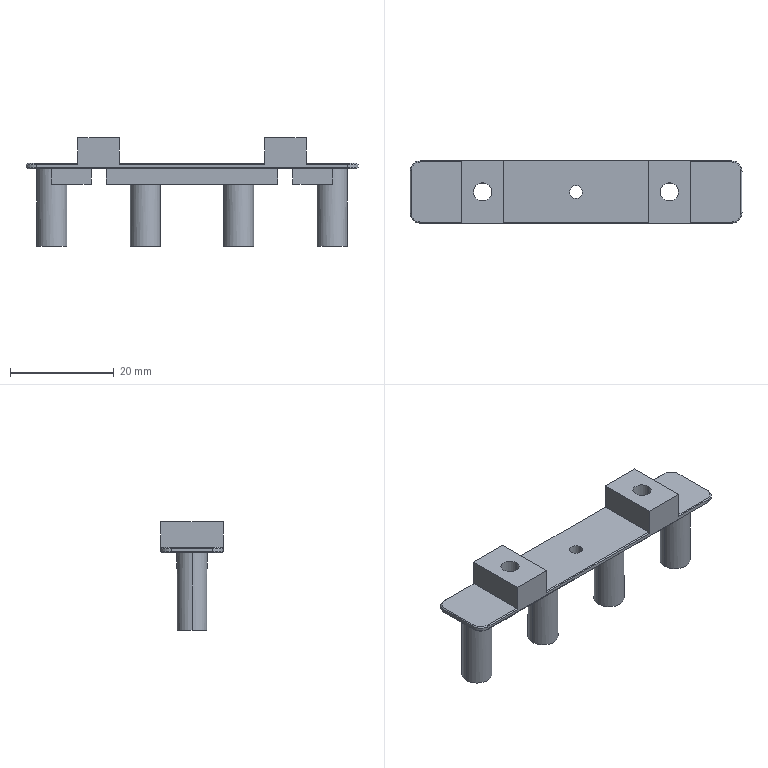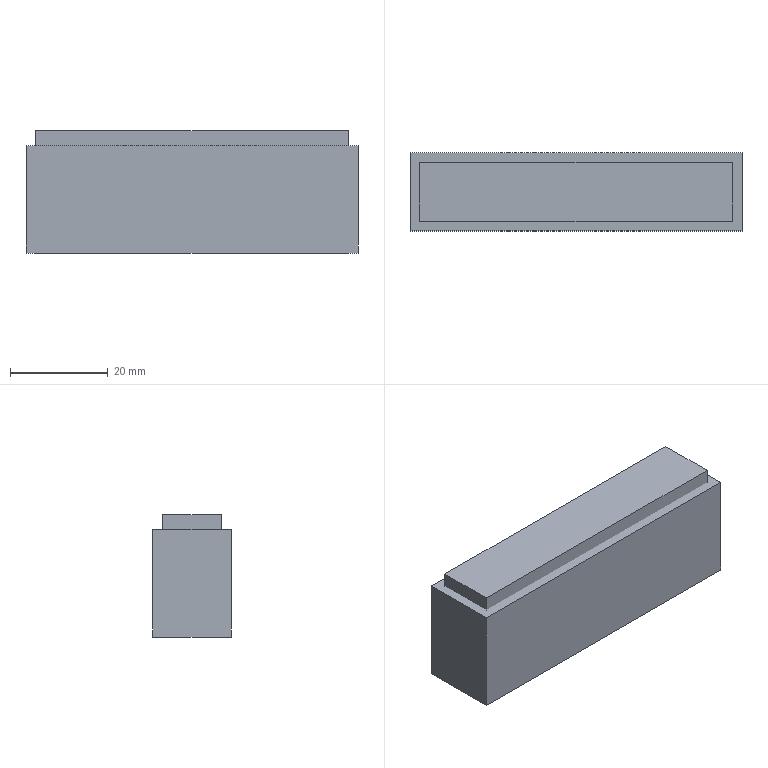CAM job | NX | 3-axis milling, drilling | part box 64 x 12 x 21 mm | stock box 68 x 16 x 25 mm
Tools:
number,name,description,diameter,corner_radius,flute_length,length,flutes
19,D80,Milling Tool-5 Parameters,80.0,0.0,50.0,75.0,2
15,D10,Milling Tool-5 Parameters,10.0,0.0,50.0,75.0,2
14,D10JING,Milling Tool-5 Parameters,10.0,0.0,50.0,75.0,2
1,D6A45,Milling Tool-5 Parameters,6.0,0.0,50.0,75.0,2
7,3.5ZT,Drilling Tool,3.5,0.0,35.0,50.0,2
2,2.5ZT,Drilling Tool,2.5,0.0,35.0,50.0,2
16,D3,Milling Tool-5 Parameters,3.0,0.0,50.0,75.0,2
12,D6,Milling Tool-5 Parameters,6.0,0.0,50.0,75.0,2
Operations:
program,operation,operation_type,tool,method,geometry_group,spindle_rpm,surface_speed,feed_per_tooth,feed_cut,feed_plunge,cut_length_mm,path_length_mm,cut_time_min,machine_time_min
1,FLOOR_WALL,VolumeBased25DMillingOperation,D80,METHOD,A,6500.0,1633.0,0.1154,1500.0,100.0,160.0,214.0,0.1067,0.1121
1,DRILLING,Operation,D6A45,METHOD,A,5000.0,94.0,0.025,250.0,0.0,12.0,126.497,0.048,0.0594
1,DRILLING_COPY,Operation,3.5ZT,METHOD,A,1910.0,21.0,0.0524,200.0,0.0,23.103,145.331,0.1155,0.1277
1,DRILLING_COPY_COPY,Operation,2.5ZT,METHOD,A,2674.0,21.0,0.028,150.0,0.0,14.251,88.502,0.095,0.1024
1,ZLEVEL_PROFILE,ZLevelMilling,D10,METHOD,A,9500.0,298.0,0.1579,3000.0,1000.0,4022.474,4100.474,1.373,1.381
1,FLOOR_WALL_1,VolumeBased25DMillingOperation,D10,METHOD,A,9500.0,298.0,0.1316,2500.0,100.0,1450.345,2184.125,0.5801,0.6535
1,ZLEVEL_PROFILE_1,ZLevelMilling,D10JING,METHOD,A,9500.0,298.0,0.0789,1500.0,1000.0,548.831,637.331,0.3673,0.3761
1,FLOOR_WALL_1_COPY,VolumeBased25DMillingOperation,D10JING,METHOD,A,9500.0,298.0,0.0789,1500.0,100.0,406.822,722.393,0.2712,0.3028
1,PLANAR_MILL_COPY_COPY_COPY,PlanarMilling,D6A45,METHOD,A,9500.0,179.0,0.0658,1250.0,100.0,120.274,407.933,0.0962,0.125
1,PLANAR_MILL_COPY_COPY_COPY_COPY,PlanarMilling,D6A45,METHOD,A,9500.0,179.0,0.0658,1250.0,100.0,119.887,444.7,0.0959,0.1284
2,FLOOR_WALL_COPY,VolumeBased25DMillingOperation,D80,METHOD,B,6500.0,1633.0,0.1154,1500.0,100.0,624.0,1278.001,0.416,0.4814
2,FLOOR_WALL_1_COPY_1,VolumeBased25DMillingOperation,D10,METHOD,B,9500.0,298.0,0.1316,2500.0,100.0,2464.512,2568.18,0.9858,0.9962
2,FLOOR_WALL_1_COPY_1_COPY,VolumeBased25DMillingOperation,D10,METHOD,B,9500.0,298.0,0.1316,2500.0,100.0,3670.675,4041.349,1.468,1.505
2,FLOOR_WALL_1_COPY_COPY,VolumeBased25DMillingOperation,D6,METHOD,B,9500.0,298.0,0.0789,1500.0,100.0,640.8,1937.456,0.4272,0.5569
2,ZLEVEL_PROFILE_COPY,ZLevelMilling,D6,METHOD,B,9500.0,298.0,0.0632,1200.0,1000.0,615.511,985.508,0.5147,0.5516
2,HOLE_MILLING,CylinderMilling,D3,METHOD,B,9500.0,89.0,0.0658,1250.0,100.0,973.65,1459.65,0.7789,0.8275
2,PLANAR_MILL_COPY_COPY_COPY_COPY_COPY,PlanarMilling,D6A45,METHOD,B,9500.0,179.0,0.0658,1250.0,100.0,155.615,244.615,0.1245,0.1334